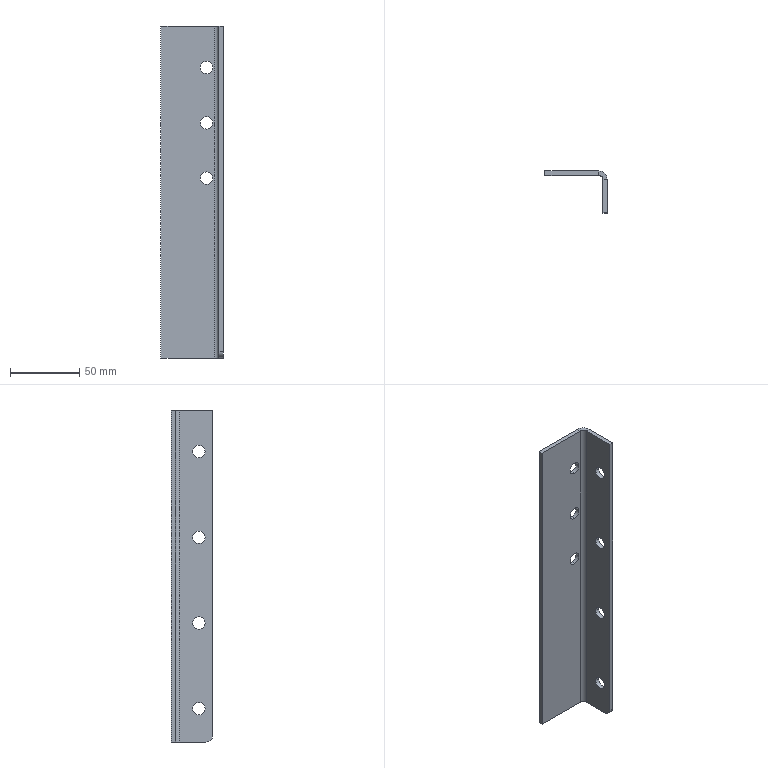Part | SolidWorks | features ICE 2, Fillet 1, FlatPattern 1, SMBaseFlange 1, SheetMetal 1 | 1 solid | 29 faces | box 45 x 30 x 240 mm | volume 49097 mm3 | cylinder 17 | plane 12 | commonest cylinder face diameters 9 x14 6 x1 10 x1 12 x1
STEP:
#1=CARTESIAN_POINT('',(33.,-3.,-25.5));
#2=VERTEX_POINT('',#1);
#3=CARTESIAN_POINT('',(33.,-3.,-34.5));
#4=VERTEX_POINT('',#3);
#5=CARTESIAN_POINT('',(33.,-3.,-30.));
#6=DIRECTION('',(0.,-1.,0.));
#7=DIRECTION('',(0.,0.,-1.));
#8=AXIS2_PLACEMENT_3D('',#5,#6,#7);
#9=CIRCLE('',#8,4.5);
#10=EDGE_CURVE('',#2,#4,#9,.T.);
#11=ORIENTED_EDGE('',*,*,#10,.T.);
#12=CARTESIAN_POINT('',(33.,0.,-34.5));
#13=VERTEX_POINT('',#12);
#14=CARTESIAN_POINT('',(33.,-10.,-34.5));
#15=DIRECTION('',(0.,1.,0.));
#16=VECTOR('',#15,1000.);
#17=LINE('',#14,#16);
#18=EDGE_CURVE('',#4,#13,#17,.T.);
#19=ORIENTED_EDGE('',*,*,#18,.T.);
#20=CARTESIAN_POINT('',(33.,0.,-25.5));
#21=VERTEX_POINT('',#20);
#22=CARTESIAN_POINT('',(33.,0.,-30.));
#23=DIRECTION('',(0.,1.,0.));
#24=DIRECTION('',(0.,0.,1.));
#25=AXIS2_PLACEMENT_3D('',#22,#23,#24);
#26=CIRCLE('',#25,4.5);
#27=EDGE_CURVE('',#13,#21,#26,.T.);
#28=ORIENTED_EDGE('',*,*,#27,.T.);
#29=CARTESIAN_POINT('',(33.,-10.,-25.5));
#30=DIRECTION('',(0.,1.,0.));
#31=VECTOR('',#30,1000.);
#32=LINE('',#29,#31);
#33=EDGE_CURVE('',#2,#21,#32,.T.);
#34=ORIENTED_EDGE('',*,*,#33,.F.);
#35=EDGE_LOOP('',(#11,#19,#28,#34));
#36=FACE_OUTER_BOUND('',#35,.T.);
#37=CARTESIAN_POINT('',(33.,-10.,-30.));
#38=DIRECTION('',(0.,1.,0.));
#39=DIRECTION('',(0.,0.,1.));
#40=AXIS2_PLACEMENT_3D('',#37,#38,#39);
#41=CYLINDRICAL_SURFACE('',#40,4.5);
#42=ADVANCED_FACE('',(#36),#41,.F.);
#43=CARTESIAN_POINT('',(33.,-3.,-65.5));
#44=VERTEX_POINT('',#43);
#45=CARTESIAN_POINT('',(33.,-3.,-74.5));
#46=VERTEX_POINT('',#45);
#47=CARTESIAN_POINT('',(33.,-3.,-70.));
#48=DIRECTION('',(0.,-1.,0.));
#49=DIRECTION('',(0.,0.,-1.));
#50=AXIS2_PLACEMENT_3D('',#47,#48,#49);
#51=CIRCLE('',#50,4.5);
#52=EDGE_CURVE('',#44,#46,#51,.T.);
#53=ORIENTED_EDGE('',*,*,#52,.T.);
#54=CARTESIAN_POINT('',(33.,0.,-74.5));
#55=VERTEX_POINT('',#54);
#56=CARTESIAN_POINT('',(33.,-10.,-74.5));
#57=DIRECTION('',(0.,1.,0.));
#58=VECTOR('',#57,1000.);
#59=LINE('',#56,#58);
#60=EDGE_CURVE('',#46,#55,#59,.T.);
#61=ORIENTED_EDGE('',*,*,#60,.T.);
#62=CARTESIAN_POINT('',(33.,0.,-65.5));
#63=VERTEX_POINT('',#62);
#64=CARTESIAN_POINT('',(33.,0.,-70.));
#65=DIRECTION('',(0.,1.,0.));
#66=DIRECTION('',(0.,0.,1.));
#67=AXIS2_PLACEMENT_3D('',#64,#65,#66);
#68=CIRCLE('',#67,4.5);
#69=EDGE_CURVE('',#55,#63,#68,.T.);
#70=ORIENTED_EDGE('',*,*,#69,.T.);
#71=CARTESIAN_POINT('',(33.,-10.,-65.5));
#72=DIRECTION('',(0.,1.,0.));
#73=VECTOR('',#72,1000.);
#74=LINE('',#71,#73);
#75=EDGE_CURVE('',#44,#63,#74,.T.);
#76=ORIENTED_EDGE('',*,*,#75,.F.);
#77=EDGE_LOOP('',(#53,#61,#70,#76));
#78=FACE_OUTER_BOUND('',#77,.T.);
#79=CARTESIAN_POINT('',(33.,-10.,-70.));
#80=DIRECTION('',(0.,1.,0.));
#81=DIRECTION('',(0.,0.,1.));
#82=AXIS2_PLACEMENT_3D('',#79,#80,#81);
#83=CYLINDRICAL_SURFACE('',#82,4.5);
#84=ADVANCED_FACE('',(#78),#83,.F.);
#85=CARTESIAN_POINT('',(33.,-3.,-105.5));
#86=VERTEX_POINT('',#85);
#87=CARTESIAN_POINT('',(33.,-3.,-114.5));
#88=VERTEX_POINT('',#87);
#89=CARTESIAN_POINT('',(33.,-3.,-110.));
#90=DIRECTION('',(0.,-1.,0.));
#91=DIRECTION('',(0.,0.,-1.));
#92=AXIS2_PLACEMENT_3D('',#89,#90,#91);
#93=CIRCLE('',#92,4.5);
#94=EDGE_CURVE('',#86,#88,#93,.T.);
#95=ORIENTED_EDGE('',*,*,#94,.T.);
#96=CARTESIAN_POINT('',(33.,0.,-114.5));
#97=VERTEX_POINT('',#96);
#98=CARTESIAN_POINT('',(33.,-10.,-114.5));
#99=DIRECTION('',(0.,1.,0.));
#100=VECTOR('',#99,1000.);
#101=LINE('',#98,#100);
#102=EDGE_CURVE('',#88,#97,#101,.T.);
#103=ORIENTED_EDGE('',*,*,#102,.T.);
#104=CARTESIAN_POINT('',(33.,0.,-105.5));
#105=VERTEX_POINT('',#104);
#106=CARTESIAN_POINT('',(33.,0.,-110.));
#107=DIRECTION('',(0.,1.,0.));
#108=DIRECTION('',(0.,0.,1.));
#109=AXIS2_PLACEMENT_3D('',#106,#107,#108);
#110=CIRCLE('',#109,4.5);
#111=EDGE_CURVE('',#97,#105,#110,.T.);
#112=ORIENTED_EDGE('',*,*,#111,.T.);
#113=CARTESIAN_POINT('',(33.,-10.,-105.5));
#114=DIRECTION('',(0.,1.,0.));
#115=VECTOR('',#114,1000.);
#116=LINE('',#113,#115);
#117=EDGE_CURVE('',#86,#105,#116,.T.);
#118=ORIENTED_EDGE('',*,*,#117,.F.);
#119=EDGE_LOOP('',(#95,#103,#112,#118));
#120=FACE_OUTER_BOUND('',#119,.T.);
#121=CARTESIAN_POINT('',(33.,-10.,-110.));
#122=DIRECTION('',(0.,1.,0.));
#123=DIRECTION('',(0.,0.,1.));
#124=AXIS2_PLACEMENT_3D('',#121,#122,#123);
#125=CYLINDRICAL_SURFACE('',#124,4.5);
#126=ADVANCED_FACE('',(#120),#125,.F.);
#127=CARTESIAN_POINT('',(42.,-15.5,-216.));
#128=VERTEX_POINT('',#127);
#129=CARTESIAN_POINT('',(42.,-24.5,-216.));
#130=VERTEX_POINT('',#129);
#131=CARTESIAN_POINT('',(42.,-20.,-216.));
#132=DIRECTION('',(-1.,0.,0.));
#133=DIRECTION('',(0.,0.,1.));
#134=AXIS2_PLACEMENT_3D('',#131,#132,#133);
#135=CIRCLE('',#134,4.5);
#136=EDGE_CURVE('',#128,#130,#135,.T.);
#137=ORIENTED_EDGE('',*,*,#136,.T.);
#138=CARTESIAN_POINT('',(45.,-24.5,-216.));
#139=VERTEX_POINT('',#138);
#140=CARTESIAN_POINT('',(0.,-24.5,-216.));
#141=DIRECTION('',(1.,0.,0.));
#142=VECTOR('',#141,1000.);
#143=LINE('',#140,#142);
#144=EDGE_CURVE('',#130,#139,#143,.T.);
#145=ORIENTED_EDGE('',*,*,#144,.T.);
#146=CARTESIAN_POINT('',(45.,-15.5,-216.));
#147=VERTEX_POINT('',#146);
#148=CARTESIAN_POINT('',(45.,-20.,-216.));
#149=DIRECTION('',(1.,0.,0.));
#150=DIRECTION('',(0.,1.,0.));
#151=AXIS2_PLACEMENT_3D('',#148,#149,#150);
#152=CIRCLE('',#151,4.5);
#153=EDGE_CURVE('',#139,#147,#152,.T.);
#154=ORIENTED_EDGE('',*,*,#153,.T.);
#155=CARTESIAN_POINT('',(0.,-15.5,-216.));
#156=DIRECTION('',(1.,0.,0.));
#157=VECTOR('',#156,1000.);
#158=LINE('',#155,#157);
#159=EDGE_CURVE('',#128,#147,#158,.T.);
#160=ORIENTED_EDGE('',*,*,#159,.F.);
#161=EDGE_LOOP('',(#137,#145,#154,#160));
#162=FACE_OUTER_BOUND('',#161,.T.);
#163=CARTESIAN_POINT('',(0.,-20.,-216.));
#164=DIRECTION('',(1.,0.,0.));
#165=DIRECTION('',(0.,1.,0.));
#166=AXIS2_PLACEMENT_3D('',#163,#164,#165);
#167=CYLINDRICAL_SURFACE('',#166,4.5);
#168=ADVANCED_FACE('',(#162),#167,.F.);
#169=CARTESIAN_POINT('',(42.,-15.5,-154.));
#170=VERTEX_POINT('',#169);
#171=CARTESIAN_POINT('',(42.,-24.5,-154.));
#172=VERTEX_POINT('',#171);
#173=CARTESIAN_POINT('',(42.,-20.,-154.));
#174=DIRECTION('',(-1.,0.,0.));
#175=DIRECTION('',(0.,0.,1.));
#176=AXIS2_PLACEMENT_3D('',#173,#174,#175);
#177=CIRCLE('',#176,4.5);
#178=EDGE_CURVE('',#170,#172,#177,.T.);
#179=ORIENTED_EDGE('',*,*,#178,.T.);
#180=CARTESIAN_POINT('',(45.,-24.5,-154.));
#181=VERTEX_POINT('',#180);
#182=CARTESIAN_POINT('',(0.,-24.5,-154.));
#183=DIRECTION('',(1.,0.,0.));
#184=VECTOR('',#183,1000.);
#185=LINE('',#182,#184);
#186=EDGE_CURVE('',#172,#181,#185,.T.);
#187=ORIENTED_EDGE('',*,*,#186,.T.);
#188=CARTESIAN_POINT('',(45.,-15.5,-154.));
#189=VERTEX_POINT('',#188);
#190=CARTESIAN_POINT('',(45.,-20.,-154.));
#191=DIRECTION('',(1.,0.,0.));
#192=DIRECTION('',(0.,1.,0.));
#193=AXIS2_PLACEMENT_3D('',#190,#191,#192);
#194=CIRCLE('',#193,4.5);
#195=EDGE_CURVE('',#181,#189,#194,.T.);
#196=ORIENTED_EDGE('',*,*,#195,.T.);
#197=CARTESIAN_POINT('',(0.,-15.5,-154.));
#198=DIRECTION('',(1.,0.,0.));
#199=VECTOR('',#198,1000.);
#200=LINE('',#197,#199);
#201=EDGE_CURVE('',#170,#189,#200,.T.);
#202=ORIENTED_EDGE('',*,*,#201,.F.);
#203=EDGE_LOOP('',(#179,#187,#196,#202));
#204=FACE_OUTER_BOUND('',#203,.T.);
#205=CARTESIAN_POINT('',(0.,-20.,-154.));
#206=DIRECTION('',(1.,0.,0.));
#207=DIRECTION('',(0.,1.,0.));
#208=AXIS2_PLACEMENT_3D('',#205,#206,#207);
#209=CYLINDRICAL_SURFACE('',#208,4.5);
#210=ADVANCED_FACE('',(#204),#209,.F.);
#211=CARTESIAN_POINT('',(42.,-15.5,-30.));
#212=VERTEX_POINT('',#211);
#213=CARTESIAN_POINT('',(42.,-24.5,-30.));
#214=VERTEX_POINT('',#213);
#215=CARTESIAN_POINT('',(42.,-20.,-30.));
#216=DIRECTION('',(-1.,0.,0.));
#217=DIRECTION('',(0.,0.,1.));
#218=AXIS2_PLACEMENT_3D('',#215,#216,#217);
#219=CIRCLE('',#218,4.5);
#220=EDGE_CURVE('',#212,#214,#219,.T.);
#221=ORIENTED_EDGE('',*,*,#220,.T.);
#222=CARTESIAN_POINT('',(45.,-24.5,-30.));
#223=VERTEX_POINT('',#222);
#224=CARTESIAN_POINT('',(0.,-24.5,-30.));
#225=DIRECTION('',(1.,0.,0.));
#226=VECTOR('',#225,1000.);
#227=LINE('',#224,#226);
#228=EDGE_CURVE('',#214,#223,#227,.T.);
#229=ORIENTED_EDGE('',*,*,#228,.T.);
#230=CARTESIAN_POINT('',(45.,-15.5,-30.));
#231=VERTEX_POINT('',#230);
#232=CARTESIAN_POINT('',(45.,-20.,-30.));
#233=DIRECTION('',(1.,0.,0.));
#234=DIRECTION('',(0.,1.,0.));
#235=AXIS2_PLACEMENT_3D('',#232,#233,#234);
#236=CIRCLE('',#235,4.5);
#237=EDGE_CURVE('',#223,#231,#236,.T.);
#238=ORIENTED_EDGE('',*,*,#237,.T.);
#239=CARTESIAN_POINT('',(0.,-15.5,-30.));
#240=DIRECTION('',(1.,0.,0.));
#241=VECTOR('',#240,1000.);
#242=LINE('',#239,#241);
#243=EDGE_CURVE('',#212,#231,#242,.T.);
#244=ORIENTED_EDGE('',*,*,#243,.F.);
#245=EDGE_LOOP('',(#221,#229,#238,#244));
#246=FACE_OUTER_BOUND('',#245,.T.);
#247=CARTESIAN_POINT('',(0.,-20.,-30.));
#248=DIRECTION('',(1.,0.,0.));
#249=DIRECTION('',(0.,1.,0.));
#250=AXIS2_PLACEMENT_3D('',#247,#248,#249);
#251=CYLINDRICAL_SURFACE('',#250,4.5);
#252=ADVANCED_FACE('',(#246),#251,.F.);
#253=CARTESIAN_POINT('',(42.,-15.5,-92.));
#254=VERTEX_POINT('',#253);
#255=CARTESIAN_POINT('',(42.,-24.5,-92.));
#256=VERTEX_POINT('',#255);
#257=CARTESIAN_POINT('',(42.,-20.,-92.));
#258=DIRECTION('',(-1.,0.,0.));
#259=DIRECTION('',(0.,0.,1.));
#260=AXIS2_PLACEMENT_3D('',#257,#258,#259);
#261=CIRCLE('',#260,4.5);
#262=EDGE_CURVE('',#254,#256,#261,.T.);
#263=ORIENTED_EDGE('',*,*,#262,.T.);
#264=CARTESIAN_POINT('',(45.,-24.5,-92.));
#265=VERTEX_POINT('',#264);
#266=CARTESIAN_POINT('',(0.,-24.5,-92.));
#267=DIRECTION('',(1.,0.,0.));
#268=VECTOR('',#267,1000.);
#269=LINE('',#266,#268);
#270=EDGE_CURVE('',#256,#265,#269,.T.);
#271=ORIENTED_EDGE('',*,*,#270,.T.);
#272=CARTESIAN_POINT('',(45.,-15.5,-92.));
#273=VERTEX_POINT('',#272);
#274=CARTESIAN_POINT('',(45.,-20.,-92.));
#275=DIRECTION('',(1.,0.,0.));
#276=DIRECTION('',(0.,1.,0.));
#277=AXIS2_PLACEMENT_3D('',#274,#275,#276);
#278=CIRCLE('',#277,4.5);
#279=EDGE_CURVE('',#265,#273,#278,.T.);
#280=ORIENTED_EDGE('',*,*,#279,.T.);
#281=CARTESIAN_POINT('',(0.,-15.5,-92.));
#282=DIRECTION('',(1.,0.,0.));
#283=VECTOR('',#282,1000.);
#284=LINE('',#281,#283);
#285=EDGE_CURVE('',#254,#273,#284,.T.);
#286=ORIENTED_EDGE('',*,*,#285,.F.);
#287=EDGE_LOOP('',(#263,#271,#280,#286));
#288=FACE_OUTER_BOUND('',#287,.T.);
#289=CARTESIAN_POINT('',(0.,-20.,-92.));
#290=DIRECTION('',(1.,0.,0.));
#291=DIRECTION('',(0.,1.,0.));
#292=AXIS2_PLACEMENT_3D('',#289,#290,#291);
#293=CYLINDRICAL_SURFACE('',#292,4.5);
#294=ADVANCED_FACE('',(#288),#293,.F.);
#295=CARTESIAN_POINT('',(45.,-25.,-240.));
#296=VERTEX_POINT('',#295);
#297=CARTESIAN_POINT('',(42.,-25.,-240.));
#298=VERTEX_POINT('',#297);
#299=CARTESIAN_POINT('',(39.,-25.,-240.));
#300=DIRECTION('',(-1.,0.,0.));
#301=VECTOR('',#300,1000.);
#302=LINE('',#299,#301);
#303=EDGE_CURVE('',#296,#298,#302,.T.);
#304=ORIENTED_EDGE('',*,*,#303,.F.);
#305=CARTESIAN_POINT('',(45.,-30.,-235.));
#306=VERTEX_POINT('',#305);
#307=CARTESIAN_POINT('',(45.,-25.,-235.));
#308=DIRECTION('',(1.,0.,0.));
#309=DIRECTION('',(0.,0.,1.));
#310=AXIS2_PLACEMENT_3D('',#307,#308,#309);
#311=CIRCLE('',#310,5.);
#312=EDGE_CURVE('',#306,#296,#311,.T.);
#313=ORIENTED_EDGE('',*,*,#312,.F.);
#314=CARTESIAN_POINT('',(42.,-30.,-235.));
#315=VERTEX_POINT('',#314);
#316=CARTESIAN_POINT('',(45.,-30.,-235.));
#317=DIRECTION('',(1.,0.,0.));
#318=VECTOR('',#317,1000.);
#319=LINE('',#316,#318);
#320=EDGE_CURVE('',#315,#306,#319,.T.);
#321=ORIENTED_EDGE('',*,*,#320,.F.);
#322=CARTESIAN_POINT('',(42.,-25.,-235.));
#323=DIRECTION('',(-1.,0.,0.));
#324=DIRECTION('',(0.,0.,1.));
#325=AXIS2_PLACEMENT_3D('',#322,#323,#324);
#326=CIRCLE('',#325,5.);
#327=EDGE_CURVE('',#298,#315,#326,.T.);
#328=ORIENTED_EDGE('',*,*,#327,.F.);
#329=EDGE_LOOP('',(#304,#313,#321,#328));
#330=FACE_OUTER_BOUND('',#329,.T.);
#331=CARTESIAN_POINT('',(39.,-25.,-235.));
#332=DIRECTION('',(-1.,0.,0.));
#333=DIRECTION('',(0.,0.,1.));
#334=AXIS2_PLACEMENT_3D('',#331,#332,#333);
#335=CYLINDRICAL_SURFACE('',#334,5.);
#336=ADVANCED_FACE('',(#330),#335,.T.);
#337=CARTESIAN_POINT('',(39.,0.,-240.));
#338=VERTEX_POINT('',#337);
#339=CARTESIAN_POINT('',(39.,-3.,-240.));
#340=VERTEX_POINT('',#339);
#341=CARTESIAN_POINT('',(39.,0.,-240.));
#342=DIRECTION('',(0.,-1.,0.));
#343=VECTOR('',#342,1000.);
#344=LINE('',#341,#343);
#345=EDGE_CURVE('',#338,#340,#344,.T.);
#346=ORIENTED_EDGE('',*,*,#345,.F.);
#347=CARTESIAN_POINT('',(45.,-6.,-240.));
#348=VERTEX_POINT('',#347);
#349=CARTESIAN_POINT('',(39.,-6.,-240.));
#350=DIRECTION('',(0.,0.,-1.));
#351=DIRECTION('',(1.,0.,0.));
#352=AXIS2_PLACEMENT_3D('',#349,#350,#351);
#353=CIRCLE('',#352,6.);
#354=EDGE_CURVE('',#338,#348,#353,.T.);
#355=ORIENTED_EDGE('',*,*,#354,.T.);
#356=CARTESIAN_POINT('',(42.,-6.,-240.));
#357=VERTEX_POINT('',#356);
#358=CARTESIAN_POINT('',(42.,-6.,-240.));
#359=DIRECTION('',(1.,0.,0.));
#360=VECTOR('',#359,1000.);
#361=LINE('',#358,#360);
#362=EDGE_CURVE('',#357,#348,#361,.T.);
#363=ORIENTED_EDGE('',*,*,#362,.F.);
#364=CARTESIAN_POINT('',(39.,-6.,-240.));
#365=DIRECTION('',(0.,0.,-1.));
#366=DIRECTION('',(1.,0.,0.));
#367=AXIS2_PLACEMENT_3D('',#364,#365,#366);
#368=CIRCLE('',#367,3.);
#369=EDGE_CURVE('',#340,#357,#368,.T.);
#370=ORIENTED_EDGE('',*,*,#369,.F.);
#371=EDGE_LOOP('',(#346,#355,#363,#370));
#372=FACE_OUTER_BOUND('',#371,.T.);
#373=CARTESIAN_POINT('',(39.,0.,-240.));
#374=DIRECTION('',(0.,0.,-1.));
#375=DIRECTION('',(-1.,0.,0.));
#376=AXIS2_PLACEMENT_3D('',#373,#374,#375);
#377=PLANE('',#376);
#378=ADVANCED_FACE('',(#372),#377,.T.);
#379=CARTESIAN_POINT('',(0.,0.,-240.));
#380=VERTEX_POINT('',#379);
#381=CARTESIAN_POINT('',(0.,0.,-240.));
#382=DIRECTION('',(1.,0.,0.));
#383=VECTOR('',#382,1000.);
#384=LINE('',#381,#383);
#385=EDGE_CURVE('',#380,#338,#384,.T.);
#386=ORIENTED_EDGE('',*,*,#385,.T.);
#387=ORIENTED_EDGE('',*,*,#345,.T.);
#388=CARTESIAN_POINT('',(0.,-3.,-240.));
#389=VERTEX_POINT('',#388);
#390=CARTESIAN_POINT('',(0.,-3.,-240.));
#391=DIRECTION('',(1.,0.,0.));
#392=VECTOR('',#391,1000.);
#393=LINE('',#390,#392);
#394=EDGE_CURVE('',#389,#340,#393,.T.);
#395=ORIENTED_EDGE('',*,*,#394,.F.);
#396=CARTESIAN_POINT('',(0.,-3.,-240.));
#397=DIRECTION('',(0.,1.,0.));
#398=VECTOR('',#397,1000.);
#399=LINE('',#396,#398);
#400=EDGE_CURVE('',#389,#380,#399,.T.);
#401=ORIENTED_EDGE('',*,*,#400,.T.);
#402=EDGE_LOOP('',(#386,#387,#395,#401));
#403=FACE_OUTER_BOUND('',#402,.T.);
#404=CARTESIAN_POINT('',(42.,-6.,-240.));
#405=DIRECTION('',(0.,0.,-1.));
#406=DIRECTION('',(-1.,0.,0.));
#407=AXIS2_PLACEMENT_3D('',#404,#405,#406);
#408=PLANE('',#407);
#409=ADVANCED_FACE('',(#403),#408,.T.);
#410=CARTESIAN_POINT('',(45.,-6.,0.));
#411=VERTEX_POINT('',#410);
#412=CARTESIAN_POINT('',(42.,-6.,0.));
#413=VERTEX_POINT('',#412);
#414=CARTESIAN_POINT('',(45.,-6.,0.));
#415=DIRECTION('',(-1.,0.,0.));
#416=VECTOR('',#415,1000.);
#417=LINE('',#414,#416);
#418=EDGE_CURVE('',#411,#413,#417,.T.);
#419=ORIENTED_EDGE('',*,*,#418,.F.);
#420=CARTESIAN_POINT('',(39.,0.,0.));
#421=VERTEX_POINT('',#420);
#422=CARTESIAN_POINT('',(39.,-6.,0.));
#423=DIRECTION('',(0.,0.,-1.));
#424=DIRECTION('',(1.,0.,0.));
#425=AXIS2_PLACEMENT_3D('',#422,#423,#424);
#426=CIRCLE('',#425,6.);
#427=EDGE_CURVE('',#421,#411,#426,.T.);
#428=ORIENTED_EDGE('',*,*,#427,.F.);
#429=CARTESIAN_POINT('',(39.,-3.,0.));
#430=VERTEX_POINT('',#429);
#431=CARTESIAN_POINT('',(39.,-3.,0.));
#432=DIRECTION('',(0.,1.,0.));
#433=VECTOR('',#432,1000.);
#434=LINE('',#431,#433);
#435=EDGE_CURVE('',#430,#421,#434,.T.);
#436=ORIENTED_EDGE('',*,*,#435,.F.);
#437=CARTESIAN_POINT('',(39.,-6.,0.));
#438=DIRECTION('',(0.,0.,-1.));
#439=DIRECTION('',(1.,0.,0.));
#440=AXIS2_PLACEMENT_3D('',#437,#438,#439);
#441=CIRCLE('',#440,3.);
#442=EDGE_CURVE('',#430,#413,#441,.T.);
#443=ORIENTED_EDGE('',*,*,#442,.T.);
#444=EDGE_LOOP('',(#419,#428,#436,#443));
#445=FACE_OUTER_BOUND('',#444,.T.);
#446=CARTESIAN_POINT('',(45.,-6.,0.));
#447=DIRECTION('',(0.,0.,1.));
#448=DIRECTION('',(1.,0.,0.));
#449=AXIS2_PLACEMENT_3D('',#446,#447,#448);
#450=PLANE('',#449);
#451=ADVANCED_FACE('',(#445),#450,.T.);
#452=CARTESIAN_POINT('',(45.,-30.,0.));
#453=VERTEX_POINT('',#452);
#454=CARTESIAN_POINT('',(45.,0.,0.));
#455=DIRECTION('',(0.,-1.,0.));
#456=VECTOR('',#455,1000.);
#457=LINE('',#454,#456);
#458=EDGE_CURVE('',#411,#453,#457,.T.);
#459=ORIENTED_EDGE('',*,*,#458,.F.);
#460=ORIENTED_EDGE('',*,*,#418,.T.);
#461=CARTESIAN_POINT('',(42.,-30.,0.));
#462=VERTEX_POINT('',#461);
#463=CARTESIAN_POINT('',(42.,0.,0.));
#464=DIRECTION('',(0.,-1.,0.));
#465=VECTOR('',#464,1000.);
#466=LINE('',#463,#465);
#467=EDGE_CURVE('',#413,#462,#466,.T.);
#468=ORIENTED_EDGE('',*,*,#467,.T.);
#469=CARTESIAN_POINT('',(45.,-30.,0.));
#470=DIRECTION('',(-1.,0.,0.));
#471=VECTOR('',#470,1000.);
#472=LINE('',#469,#471);
#473=EDGE_CURVE('',#453,#462,#472,.T.);
#474=ORIENTED_EDGE('',*,*,#473,.F.);
#475=EDGE_LOOP('',(#459,#460,#468,#474));
#476=FACE_OUTER_BOUND('',#475,.T.);
#477=CARTESIAN_POINT('',(39.,-3.,0.));
#478=DIRECTION('',(0.,0.,1.));
#479=DIRECTION('',(1.,0.,0.));
#480=AXIS2_PLACEMENT_3D('',#477,#478,#479);
#481=PLANE('',#480);
#482=ADVANCED_FACE('',(#476),#481,.T.);
#483=ORIENTED_EDGE('',*,*,#136,.F.);
#484=CARTESIAN_POINT('',(42.,-20.,-216.));
#485=DIRECTION('',(-1.,0.,0.));
#486=DIRECTION('',(0.,0.,1.));
#487=AXIS2_PLACEMENT_3D('',#484,#485,#486);
#488=CIRCLE('',#487,4.5);
#489=EDGE_CURVE('',#130,#128,#488,.T.);
#490=ORIENTED_EDGE('',*,*,#489,.F.);
#491=EDGE_LOOP('',(#483,#490));
#492=FACE_BOUND('',#491,.T.);
#493=ORIENTED_EDGE('',*,*,#178,.F.);
#494=CARTESIAN_POINT('',(42.,-20.,-154.));
#495=DIRECTION('',(-1.,0.,0.));
#496=DIRECTION('',(0.,0.,1.));
#497=AXIS2_PLACEMENT_3D('',#494,#495,#496);
#498=CIRCLE('',#497,4.5);
#499=EDGE_CURVE('',#172,#170,#498,.T.);
#500=ORIENTED_EDGE('',*,*,#499,.F.);
#501=EDGE_LOOP('',(#493,#500));
#502=FACE_BOUND('',#501,.T.);
#503=ORIENTED_EDGE('',*,*,#220,.F.);
#504=CARTESIAN_POINT('',(42.,-20.,-30.));
#505=DIRECTION('',(-1.,0.,0.));
#506=DIRECTION('',(0.,0.,1.));
#507=AXIS2_PLACEMENT_3D('',#504,#505,#506);
#508=CIRCLE('',#507,4.5);
#509=EDGE_CURVE('',#214,#212,#508,.T.);
#510=ORIENTED_EDGE('',*,*,#509,.F.);
#511=EDGE_LOOP('',(#503,#510));
#512=FACE_BOUND('',#511,.T.);
#513=ORIENTED_EDGE('',*,*,#262,.F.);
#514=CARTESIAN_POINT('',(42.,-20.,-92.));
#515=DIRECTION('',(-1.,0.,0.));
#516=DIRECTION('',(0.,0.,1.));
#517=AXIS2_PLACEMENT_3D('',#514,#515,#516);
#518=CIRCLE('',#517,4.5);
#519=EDGE_CURVE('',#256,#254,#518,.T.);
#520=ORIENTED_EDGE('',*,*,#519,.F.);
#521=EDGE_LOOP('',(#513,#520));
#522=FACE_BOUND('',#521,.T.);
#523=CARTESIAN_POINT('',(42.,0.,-240.));
#524=DIRECTION('',(0.,-1.,0.));
#525=VECTOR('',#524,1000.);
#526=LINE('',#523,#525);
#527=EDGE_CURVE('',#357,#298,#526,.T.);
#528=ORIENTED_EDGE('',*,*,#527,.T.);
#529=ORIENTED_EDGE('',*,*,#327,.T.);
#530=CARTESIAN_POINT('',(42.,-30.,-240.));
#531=DIRECTION('',(0.,0.,1.));
#532=VECTOR('',#531,1000.);
#533=LINE('',#530,#532);
#534=EDGE_CURVE('',#315,#462,#533,.T.);
#535=ORIENTED_EDGE('',*,*,#534,.T.);
#536=ORIENTED_EDGE('',*,*,#467,.F.);
#537=CARTESIAN_POINT('',(42.,-6.,-240.));
#538=DIRECTION('',(0.,0.,1.));
#539=VECTOR('',#538,1000.);
#540=LINE('',#537,#539);
#541=EDGE_CURVE('',#357,#413,#540,.T.);
#542=ORIENTED_EDGE('',*,*,#541,.F.);
#543=EDGE_LOOP('',(#528,#529,#535,#536,#542));
#544=FACE_OUTER_BOUND('',#543,.T.);
#545=CARTESIAN_POINT('',(42.,0.,-240.));
#546=DIRECTION('',(-1.,0.,0.));
#547=DIRECTION('',(0.,0.,1.));
#548=AXIS2_PLACEMENT_3D('',#545,#546,#547);
#549=PLANE('',#548);
#550=ADVANCED_FACE('',(#492,#502,#512,#522,#544),#549,.T.);
#551=ORIENTED_EDGE('',*,*,#442,.F.);
#552=CARTESIAN_POINT('',(39.,-3.,-240.));
#553=DIRECTION('',(0.,0.,1.));
#554=VECTOR('',#553,1000.);
#555=LINE('',#552,#554);
#556=EDGE_CURVE('',#340,#430,#555,.T.);
#557=ORIENTED_EDGE('',*,*,#556,.F.);
#558=ORIENTED_EDGE('',*,*,#369,.T.);
#559=ORIENTED_EDGE('',*,*,#541,.T.);
#560=EDGE_LOOP('',(#551,#557,#558,#559));
#561=FACE_OUTER_BOUND('',#560,.T.);
#562=CARTESIAN_POINT('',(39.,-6.,-240.));
#563=DIRECTION('',(0.,0.,1.));
#564=DIRECTION('',(1.,0.,0.));
#565=AXIS2_PLACEMENT_3D('',#562,#563,#564);
#566=CYLINDRICAL_SURFACE('',#565,3.);
#567=ADVANCED_FACE('',(#561),#566,.F.);
#568=ORIENTED_EDGE('',*,*,#10,.F.);
#569=CARTESIAN_POINT('',(33.,-3.,-30.));
#570=DIRECTION('',(0.,-1.,0.));
#571=DIRECTION('',(0.,0.,-1.));
#572=AXIS2_PLACEMENT_3D('',#569,#570,#571);
#573=CIRCLE('',#572,4.5);
#574=EDGE_CURVE('',#4,#2,#573,.T.);
#575=ORIENTED_EDGE('',*,*,#574,.F.);
#576=EDGE_LOOP('',(#568,#575));
#577=FACE_BOUND('',#576,.T.);
#578=ORIENTED_EDGE('',*,*,#52,.F.);
#579=CARTESIAN_POINT('',(33.,-3.,-70.));
#580=DIRECTION('',(0.,-1.,0.));
#581=DIRECTION('',(0.,0.,-1.));
#582=AXIS2_PLACEMENT_3D('',#579,#580,#581);
#583=CIRCLE('',#582,4.5);
#584=EDGE_CURVE('',#46,#44,#583,.T.);
#585=ORIENTED_EDGE('',*,*,#584,.F.);
#586=EDGE_LOOP('',(#578,#585));
#587=FACE_BOUND('',#586,.T.);
#588=ORIENTED_EDGE('',*,*,#94,.F.);
#589=CARTESIAN_POINT('',(33.,-3.,-110.));
#590=DIRECTION('',(0.,-1.,0.));
#591=DIRECTION('',(0.,0.,-1.));
#592=AXIS2_PLACEMENT_3D('',#589,#590,#591);
#593=CIRCLE('',#592,4.5);
#594=EDGE_CURVE('',#88,#86,#593,.T.);
#595=ORIENTED_EDGE('',*,*,#594,.F.);
#596=EDGE_LOOP('',(#588,#595));
#597=FACE_BOUND('',#596,.T.);
#598=CARTESIAN_POINT('',(0.,-3.,0.));
#599=VERTEX_POINT('',#598);
#600=CARTESIAN_POINT('',(0.,-3.,0.));
#601=DIRECTION('',(1.,0.,0.));
#602=VECTOR('',#601,1000.);
#603=LINE('',#600,#602);
#604=EDGE_CURVE('',#599,#430,#603,.T.);
#605=ORIENTED_EDGE('',*,*,#604,.F.);
#606=CARTESIAN_POINT('',(0.,-3.,-240.));
#607=DIRECTION('',(0.,0.,1.));
#608=VECTOR('',#607,1000.);
#609=LINE('',#606,#608);
#610=EDGE_CURVE('',#389,#599,#609,.T.);
#611=ORIENTED_EDGE('',*,*,#610,.F.);
#612=ORIENTED_EDGE('',*,*,#394,.T.);
#613=ORIENTED_EDGE('',*,*,#556,.T.);
#614=EDGE_LOOP('',(#605,#611,#612,#613));
#615=FACE_OUTER_BOUND('',#614,.T.);
#616=CARTESIAN_POINT('',(0.,-3.,-240.));
#617=DIRECTION('',(0.,-1.,0.));
#618=DIRECTION('',(0.,0.,-1.));
#619=AXIS2_PLACEMENT_3D('',#616,#617,#618);
#620=PLANE('',#619);
#621=ADVANCED_FACE('',(#577,#587,#597,#615),#620,.T.);
#622=CARTESIAN_POINT('',(0.,0.,0.));
#623=VERTEX_POINT('',#622);
#624=CARTESIAN_POINT('',(0.,-3.,0.));
#625=DIRECTION('',(0.,1.,0.));
#626=VECTOR('',#625,1000.);
#627=LINE('',#624,#626);
#628=EDGE_CURVE('',#599,#623,#627,.T.);
#629=ORIENTED_EDGE('',*,*,#628,.T.);
#630=CARTESIAN_POINT('',(0.,0.,-240.));
#631=DIRECTION('',(0.,0.,1.));
#632=VECTOR('',#631,1000.);
#633=LINE('',#630,#632);
#634=EDGE_CURVE('',#380,#623,#633,.T.);
#635=ORIENTED_EDGE('',*,*,#634,.F.);
#636=ORIENTED_EDGE('',*,*,#400,.F.);
#637=ORIENTED_EDGE('',*,*,#610,.T.);
#638=EDGE_LOOP('',(#629,#635,#636,#637));
#639=FACE_OUTER_BOUND('',#638,.T.);
#640=CARTESIAN_POINT('',(0.,-3.,-240.));
#641=DIRECTION('',(1.,0.,0.));
#642=DIRECTION('',(0.,0.,-1.));
#643=AXIS2_PLACEMENT_3D('',#640,#641,#642);
#644=PLANE('',#643);
#645=ADVANCED_FACE('',(#639),#644,.F.);
#646=CARTESIAN_POINT('',(33.,0.,-30.));
#647=DIRECTION('',(0.,1.,0.));
#648=DIRECTION('',(0.,0.,1.));
#649=AXIS2_PLACEMENT_3D('',#646,#647,#648);
#650=CIRCLE('',#649,4.5);
#651=EDGE_CURVE('',#21,#13,#650,.T.);
#652=ORIENTED_EDGE('',*,*,#651,.F.);
#653=ORIENTED_EDGE('',*,*,#27,.F.);
#654=EDGE_LOOP('',(#652,#653));
#655=FACE_BOUND('',#654,.T.);
#656=CARTESIAN_POINT('',(33.,0.,-70.));
#657=DIRECTION('',(0.,1.,0.));
#658=DIRECTION('',(0.,0.,1.));
#659=AXIS2_PLACEMENT_3D('',#656,#657,#658);
#660=CIRCLE('',#659,4.5);
#661=EDGE_CURVE('',#63,#55,#660,.T.);
#662=ORIENTED_EDGE('',*,*,#661,.F.);
#663=ORIENTED_EDGE('',*,*,#69,.F.);
#664=EDGE_LOOP('',(#662,#663));
#665=FACE_BOUND('',#664,.T.);
#666=CARTESIAN_POINT('',(33.,0.,-110.));
#667=DIRECTION('',(0.,1.,0.));
#668=DIRECTION('',(0.,0.,1.));
#669=AXIS2_PLACEMENT_3D('',#666,#667,#668);
#670=CIRCLE('',#669,4.5);
#671=EDGE_CURVE('',#105,#97,#670,.T.);
#672=ORIENTED_EDGE('',*,*,#671,.F.);
#673=ORIENTED_EDGE('',*,*,#111,.F.);
#674=EDGE_LOOP('',(#672,#673));
#675=FACE_BOUND('',#674,.T.);
#676=CARTESIAN_POINT('',(0.,0.,0.));
#677=DIRECTION('',(1.,0.,0.));
#678=VECTOR('',#677,1000.);
#679=LINE('',#676,#678);
#680=EDGE_CURVE('',#623,#421,#679,.T.);
#681=ORIENTED_EDGE('',*,*,#680,.T.);
#682=CARTESIAN_POINT('',(39.,0.,-240.));
#683=DIRECTION('',(0.,0.,1.));
#684=VECTOR('',#683,1000.);
#685=LINE('',#682,#684);
#686=EDGE_CURVE('',#338,#421,#685,.T.);
#687=ORIENTED_EDGE('',*,*,#686,.F.);
#688=ORIENTED_EDGE('',*,*,#385,.F.);
#689=ORIENTED_EDGE('',*,*,#634,.T.);
#690=EDGE_LOOP('',(#681,#687,#688,#689));
#691=FACE_OUTER_BOUND('',#690,.T.);
#692=CARTESIAN_POINT('',(0.,0.,-240.));
#693=DIRECTION('',(0.,-1.,0.));
#694=DIRECTION('',(0.,0.,-1.));
#695=AXIS2_PLACEMENT_3D('',#692,#693,#694);
#696=PLANE('',#695);
#697=ADVANCED_FACE('',(#655,#665,#675,#691),#696,.F.);
#698=ORIENTED_EDGE('',*,*,#427,.T.);
#699=CARTESIAN_POINT('',(45.,-6.,-240.));
#700=DIRECTION('',(0.,0.,1.));
#701=VECTOR('',#700,1000.);
#702=LINE('',#699,#701);
#703=EDGE_CURVE('',#348,#411,#702,.T.);
#704=ORIENTED_EDGE('',*,*,#703,.F.);
#705=ORIENTED_EDGE('',*,*,#354,.F.);
#706=ORIENTED_EDGE('',*,*,#686,.T.);
#707=EDGE_LOOP('',(#698,#704,#705,#706));
#708=FACE_OUTER_BOUND('',#707,.T.);
#709=CARTESIAN_POINT('',(39.,-6.,-240.));
#710=DIRECTION('',(0.,0.,1.));
#711=DIRECTION('',(1.,0.,0.));
#712=AXIS2_PLACEMENT_3D('',#709,#710,#711);
#713=CYLINDRICAL_SURFACE('',#712,6.);
#714=ADVANCED_FACE('',(#708),#713,.T.);
#715=CARTESIAN_POINT('',(45.,-20.,-216.));
#716=DIRECTION('',(1.,0.,0.));
#717=DIRECTION('',(0.,1.,0.));
#718=AXIS2_PLACEMENT_3D('',#715,#716,#717);
#719=CIRCLE('',#718,4.5);
#720=EDGE_CURVE('',#147,#139,#719,.T.);
#721=ORIENTED_EDGE('',*,*,#720,.F.);
#722=ORIENTED_EDGE('',*,*,#153,.F.);
#723=EDGE_LOOP('',(#721,#722));
#724=FACE_BOUND('',#723,.T.);
#725=CARTESIAN_POINT('',(45.,-20.,-154.));
#726=DIRECTION('',(1.,0.,0.));
#727=DIRECTION('',(0.,1.,0.));
#728=AXIS2_PLACEMENT_3D('',#725,#726,#727);
#729=CIRCLE('',#728,4.5);
#730=EDGE_CURVE('',#189,#181,#729,.T.);
#731=ORIENTED_EDGE('',*,*,#730,.F.);
#732=ORIENTED_EDGE('',*,*,#195,.F.);
#733=EDGE_LOOP('',(#731,#732));
#734=FACE_BOUND('',#733,.T.);
#735=CARTESIAN_POINT('',(45.,-20.,-30.));
#736=DIRECTION('',(1.,0.,0.));
#737=DIRECTION('',(0.,1.,0.));
#738=AXIS2_PLACEMENT_3D('',#735,#736,#737);
#739=CIRCLE('',#738,4.5);
#740=EDGE_CURVE('',#231,#223,#739,.T.);
#741=ORIENTED_EDGE('',*,*,#740,.F.);
#742=ORIENTED_EDGE('',*,*,#237,.F.);
#743=EDGE_LOOP('',(#741,#742));
#744=FACE_BOUND('',#743,.T.);
#745=CARTESIAN_POINT('',(45.,-20.,-92.));
#746=DIRECTION('',(1.,0.,0.));
#747=DIRECTION('',(0.,1.,0.));
#748=AXIS2_PLACEMENT_3D('',#745,#746,#747);
#749=CIRCLE('',#748,4.5);
#750=EDGE_CURVE('',#273,#265,#749,.T.);
#751=ORIENTED_EDGE('',*,*,#750,.F.);
#752=ORIENTED_EDGE('',*,*,#279,.F.);
#753=EDGE_LOOP('',(#751,#752));
#754=FACE_BOUND('',#753,.T.);
#755=CARTESIAN_POINT('',(45.,-30.,-240.));
#756=DIRECTION('',(0.,0.,1.));
#757=VECTOR('',#756,1000.);
#758=LINE('',#755,#757);
#759=EDGE_CURVE('',#306,#453,#758,.T.);
#760=ORIENTED_EDGE('',*,*,#759,.F.);
#761=ORIENTED_EDGE('',*,*,#312,.T.);
#762=CARTESIAN_POINT('',(45.,0.,-240.));
#763=DIRECTION('',(0.,-1.,0.));
#764=VECTOR('',#763,1000.);
#765=LINE('',#762,#764);
#766=EDGE_CURVE('',#348,#296,#765,.T.);
#767=ORIENTED_EDGE('',*,*,#766,.F.);
#768=ORIENTED_EDGE('',*,*,#703,.T.);
#769=ORIENTED_EDGE('',*,*,#458,.T.);
#770=EDGE_LOOP('',(#760,#761,#767,#768,#769));
#771=FACE_OUTER_BOUND('',#770,.T.);
#772=CARTESIAN_POINT('',(45.,0.,-240.));
#773=DIRECTION('',(-1.,0.,0.));
#774=DIRECTION('',(0.,0.,1.));
#775=AXIS2_PLACEMENT_3D('',#772,#773,#774);
#776=PLANE('',#775);
#777=ADVANCED_FACE('',(#724,#734,#744,#754,#771),#776,.F.);
#778=ORIENTED_EDGE('',*,*,#534,.F.);
#779=ORIENTED_EDGE('',*,*,#320,.T.);
#780=ORIENTED_EDGE('',*,*,#759,.T.);
#781=ORIENTED_EDGE('',*,*,#473,.T.);
#782=EDGE_LOOP('',(#778,#779,#780,#781));
#783=FACE_OUTER_BOUND('',#782,.T.);
#784=CARTESIAN_POINT('',(45.,-30.,-240.));
#785=DIRECTION('',(0.,1.,0.));
#786=DIRECTION('',(0.,0.,1.));
#787=AXIS2_PLACEMENT_3D('',#784,#785,#786);
#788=PLANE('',#787);
#789=ADVANCED_FACE('',(#783),#788,.F.);
#790=ORIENTED_EDGE('',*,*,#766,.T.);
#791=ORIENTED_EDGE('',*,*,#303,.T.);
#792=ORIENTED_EDGE('',*,*,#527,.F.);
#793=ORIENTED_EDGE('',*,*,#362,.T.);
#794=EDGE_LOOP('',(#790,#791,#792,#793));
#795=FACE_OUTER_BOUND('',#794,.T.);
#796=CARTESIAN_POINT('',(39.,-6.,-240.));
#797=DIRECTION('',(0.,0.,1.));
#798=DIRECTION('',(1.,0.,0.));
#799=AXIS2_PLACEMENT_3D('',#796,#797,#798);
#800=PLANE('',#799);
#801=ADVANCED_FACE('',(#795),#800,.F.);
#802=ORIENTED_EDGE('',*,*,#604,.T.);
#803=ORIENTED_EDGE('',*,*,#435,.T.);
#804=ORIENTED_EDGE('',*,*,#680,.F.);
#805=ORIENTED_EDGE('',*,*,#628,.F.);
#806=EDGE_LOOP('',(#802,#803,#804,#805));
#807=FACE_OUTER_BOUND('',#806,.T.);
#808=CARTESIAN_POINT('',(39.,-6.,0.));
#809=DIRECTION('',(0.,0.,1.));
#810=DIRECTION('',(1.,0.,0.));
#811=AXIS2_PLACEMENT_3D('',#808,#809,#810);
#812=PLANE('',#811);
#813=ADVANCED_FACE('',(#807),#812,.T.);
#814=ORIENTED_EDGE('',*,*,#270,.F.);
#815=ORIENTED_EDGE('',*,*,#519,.T.);
#816=ORIENTED_EDGE('',*,*,#285,.T.);
#817=ORIENTED_EDGE('',*,*,#750,.T.);
#818=EDGE_LOOP('',(#814,#815,#816,#817));
#819=FACE_OUTER_BOUND('',#818,.T.);
#820=CARTESIAN_POINT('',(0.,-20.,-92.));
#821=DIRECTION('',(1.,0.,0.));
#822=DIRECTION('',(0.,1.,0.));
#823=AXIS2_PLACEMENT_3D('',#820,#821,#822);
#824=CYLINDRICAL_SURFACE('',#823,4.5);
#825=ADVANCED_FACE('',(#819),#824,.F.);
#826=ORIENTED_EDGE('',*,*,#228,.F.);
#827=ORIENTED_EDGE('',*,*,#509,.T.);
#828=ORIENTED_EDGE('',*,*,#243,.T.);
#829=ORIENTED_EDGE('',*,*,#740,.T.);
#830=EDGE_LOOP('',(#826,#827,#828,#829));
#831=FACE_OUTER_BOUND('',#830,.T.);
#832=CARTESIAN_POINT('',(0.,-20.,-30.));
#833=DIRECTION('',(1.,0.,0.));
#834=DIRECTION('',(0.,1.,0.));
#835=AXIS2_PLACEMENT_3D('',#832,#833,#834);
#836=CYLINDRICAL_SURFACE('',#835,4.5);
#837=ADVANCED_FACE('',(#831),#836,.F.);
#838=ORIENTED_EDGE('',*,*,#186,.F.);
#839=ORIENTED_EDGE('',*,*,#499,.T.);
#840=ORIENTED_EDGE('',*,*,#201,.T.);
#841=ORIENTED_EDGE('',*,*,#730,.T.);
#842=EDGE_LOOP('',(#838,#839,#840,#841));
#843=FACE_OUTER_BOUND('',#842,.T.);
#844=CARTESIAN_POINT('',(0.,-20.,-154.));
#845=DIRECTION('',(1.,0.,0.));
#846=DIRECTION('',(0.,1.,0.));
#847=AXIS2_PLACEMENT_3D('',#844,#845,#846);
#848=CYLINDRICAL_SURFACE('',#847,4.5);
#849=ADVANCED_FACE('',(#843),#848,.F.);
#850=ORIENTED_EDGE('',*,*,#144,.F.);
#851=ORIENTED_EDGE('',*,*,#489,.T.);
#852=ORIENTED_EDGE('',*,*,#159,.T.);
#853=ORIENTED_EDGE('',*,*,#720,.T.);
#854=EDGE_LOOP('',(#850,#851,#852,#853));
#855=FACE_OUTER_BOUND('',#854,.T.);
#856=CARTESIAN_POINT('',(0.,-20.,-216.));
#857=DIRECTION('',(1.,0.,0.));
#858=DIRECTION('',(0.,1.,0.));
#859=AXIS2_PLACEMENT_3D('',#856,#857,#858);
#860=CYLINDRICAL_SURFACE('',#859,4.5);
#861=ADVANCED_FACE('',(#855),#860,.F.);
#862=ORIENTED_EDGE('',*,*,#102,.F.);
#863=ORIENTED_EDGE('',*,*,#594,.T.);
#864=ORIENTED_EDGE('',*,*,#117,.T.);
#865=ORIENTED_EDGE('',*,*,#671,.T.);
#866=EDGE_LOOP('',(#862,#863,#864,#865));
#867=FACE_OUTER_BOUND('',#866,.T.);
#868=CARTESIAN_POINT('',(33.,-10.,-110.));
#869=DIRECTION('',(0.,1.,0.));
#870=DIRECTION('',(0.,0.,1.));
#871=AXIS2_PLACEMENT_3D('',#868,#869,#870);
#872=CYLINDRICAL_SURFACE('',#871,4.5);
#873=ADVANCED_FACE('',(#867),#872,.F.);
#874=ORIENTED_EDGE('',*,*,#60,.F.);
#875=ORIENTED_EDGE('',*,*,#584,.T.);
#876=ORIENTED_EDGE('',*,*,#75,.T.);
#877=ORIENTED_EDGE('',*,*,#661,.T.);
#878=EDGE_LOOP('',(#874,#875,#876,#877));
#879=FACE_OUTER_BOUND('',#878,.T.);
#880=CARTESIAN_POINT('',(33.,-10.,-70.));
#881=DIRECTION('',(0.,1.,0.));
#882=DIRECTION('',(0.,0.,1.));
#883=AXIS2_PLACEMENT_3D('',#880,#881,#882);
#884=CYLINDRICAL_SURFACE('',#883,4.5);
#885=ADVANCED_FACE('',(#879),#884,.F.);
#886=ORIENTED_EDGE('',*,*,#18,.F.);
#887=ORIENTED_EDGE('',*,*,#574,.T.);
#888=ORIENTED_EDGE('',*,*,#33,.T.);
#889=ORIENTED_EDGE('',*,*,#651,.T.);
#890=EDGE_LOOP('',(#886,#887,#888,#889));
#891=FACE_OUTER_BOUND('',#890,.T.);
#892=CARTESIAN_POINT('',(33.,-10.,-30.));
#893=DIRECTION('',(0.,1.,0.));
#894=DIRECTION('',(0.,0.,1.));
#895=AXIS2_PLACEMENT_3D('',#892,#893,#894);
#896=CYLINDRICAL_SURFACE('',#895,4.5);
#897=ADVANCED_FACE('',(#891),#896,.F.);
#898=CLOSED_SHELL('',(#42,#84,#126,#168,#210,#252,#294,#336,#378,#409,#451,#482,#550,#567,#621,#645,#697,#714,#777,#789,#801,#813,#825,#837,#849,#861,#873,#885,#897));
#899=MANIFOLD_SOLID_BREP('',#898);
#900=CARTESIAN_POINT('',(0.,0.,0.));
#901=DIRECTION('',(0.,0.,1.));
#902=DIRECTION('',(1.,0.,0.));
#903=AXIS2_PLACEMENT_3D('',#900,#901,#902);
#904=(LENGTH_UNIT()NAMED_UNIT(*)SI_UNIT(.MILLI.,.METRE.));
#905=UNCERTAINTY_MEASURE_WITH_UNIT(LENGTH_MEASURE(0.00001),#904,'','');
#906=(NAMED_UNIT(*)PLANE_ANGLE_UNIT()SI_UNIT($,.RADIAN.));
#907=(NAMED_UNIT(*)SI_UNIT($,.STERADIAN.)SOLID_ANGLE_UNIT());
#908=(GEOMETRIC_REPRESENTATION_CONTEXT(3)GLOBAL_UNCERTAINTY_ASSIGNED_CONTEXT((#905))GLOBAL_UNIT_ASSIGNED_CONTEXT((#904,#906,#907))REPRESENTATION_CONTEXT('',''));
#909=ADVANCED_BREP_SHAPE_REPRESENTATION('',(#899,#903),#908);